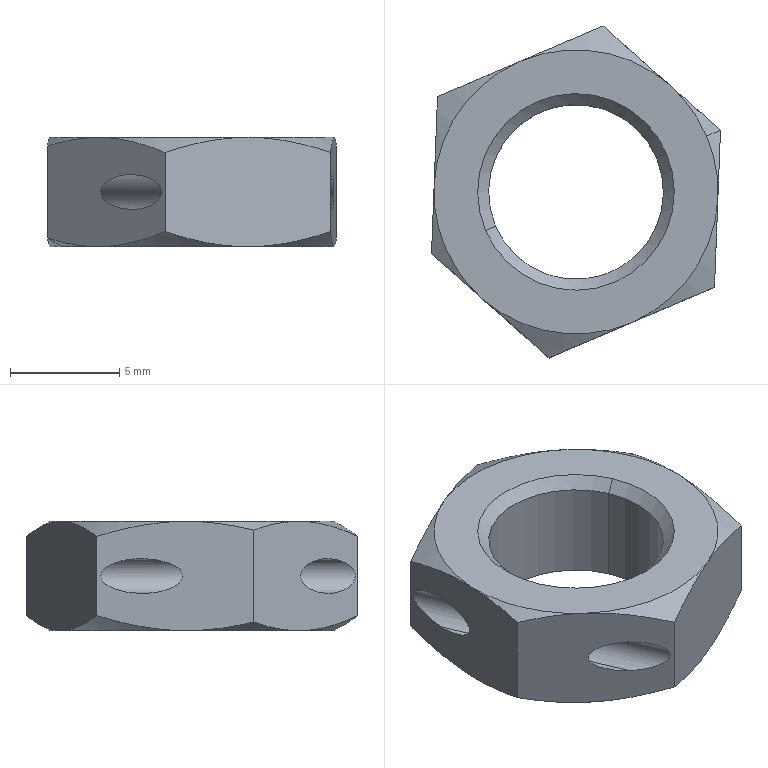Part | SolidWorks | features BaseBody 1 | 1 solid | 30 faces | box 13.225 x 15.189 x 5 mm | volume 437.577 mm3 | cone 16 | plane 8 | cylinder 6 | commonest cylinder face diameters 1.6 x4 8 x2
STEP:
#1=CARTESIAN_POINT('',(8.515,30.449,-145.05));
#2=VERTEX_POINT('',#1);
#3=CARTESIAN_POINT('',(6.902,32.713,-145.05));
#4=VERTEX_POINT('',#3);
#5=CARTESIAN_POINT('',(2.537,27.896,-145.05));
#6=DIRECTION('',(0.,0.,1.));
#7=DIRECTION('',(-0.9196,-0.3927,0.));
#8=AXIS2_PLACEMENT_3D('',#5,#6,#7);
#9=CIRCLE('',#8,6.5);
#10=EDGE_CURVE('',#2,#4,#9,.T.);
#11=ORIENTED_EDGE('',*,*,#10,.F.);
#12=CARTESIAN_POINT('',(9.149,30.72,-145.448));
#13=VERTEX_POINT('',#12);
#14=CARTESIAN_POINT('',(8.515,30.449,-145.05));
#15=DIRECTION('',(0.7964,0.3401,-0.5));
#16=VECTOR('',#15,1000.);
#17=LINE('',#14,#16);
#18=EDGE_CURVE('',#2,#13,#17,.T.);
#19=ORIENTED_EDGE('',*,*,#18,.T.);
#20=CARTESIAN_POINT('',(9.149,30.72,-145.448));
#21=CARTESIAN_POINT('',(8.411,31.375,-145.205));
#22=CARTESIAN_POINT('',(7.664,32.038,-145.056));
#23=CARTESIAN_POINT('',(6.902,32.713,-145.05));
#24=B_SPLINE_CURVE_WITH_KNOTS('',3,(#20,#21,#22,#23),.UNSPECIFIED.,.F.,.F.,(4,4),(0.,0.00303),.UNSPECIFIED.);
#25=EDGE_CURVE('',#13,#4,#24,.T.);
#26=ORIENTED_EDGE('',*,*,#25,.T.);
#27=EDGE_LOOP('',(#11,#19,#26));
#28=FACE_OUTER_BOUND('',#27,.T.);
#29=CARTESIAN_POINT('',(2.537,27.896,-145.05));
#30=DIRECTION('',(0.,0.,-1.));
#31=DIRECTION('',(0.9196,0.3927,0.));
#32=AXIS2_PLACEMENT_3D('',#29,#30,#31);
#33=CONICAL_SURFACE('',#32,6.5,1.047);
#34=ADVANCED_FACE('',(#28),#33,.T.);
#35=CARTESIAN_POINT('',(-3.958,28.144,-150.05));
#36=VERTEX_POINT('',#35);
#37=CARTESIAN_POINT('',(-3.441,25.343,-150.05));
#38=VERTEX_POINT('',#37);
#39=CARTESIAN_POINT('',(2.537,27.896,-150.05));
#40=DIRECTION('',(0.,0.,1.));
#41=DIRECTION('',(-0.9196,-0.3927,0.));
#42=AXIS2_PLACEMENT_3D('',#39,#40,#41);
#43=CIRCLE('',#42,6.5);
#44=EDGE_CURVE('',#36,#38,#43,.T.);
#45=ORIENTED_EDGE('',*,*,#44,.T.);
#46=CARTESIAN_POINT('',(-4.075,25.072,-149.652));
#47=VERTEX_POINT('',#46);
#48=CARTESIAN_POINT('',(-3.441,25.343,-150.05));
#49=DIRECTION('',(-0.7964,-0.3401,0.5));
#50=VECTOR('',#49,1000.);
#51=LINE('',#48,#50);
#52=EDGE_CURVE('',#38,#47,#51,.T.);
#53=ORIENTED_EDGE('',*,*,#52,.T.);
#54=CARTESIAN_POINT('',(-4.075,25.072,-149.652));
#55=CARTESIAN_POINT('',(-4.037,26.081,-149.901));
#56=CARTESIAN_POINT('',(-3.998,27.103,-150.05));
#57=CARTESIAN_POINT('',(-3.958,28.144,-150.05));
#58=B_SPLINE_CURVE_WITH_KNOTS('',3,(#54,#55,#56,#57),.UNSPECIFIED.,.F.,.F.,(4,4),(0.,0.003099),.UNSPECIFIED.);
#59=EDGE_CURVE('',#47,#36,#58,.T.);
#60=ORIENTED_EDGE('',*,*,#59,.T.);
#61=EDGE_LOOP('',(#45,#53,#60));
#62=FACE_OUTER_BOUND('',#61,.T.);
#63=CARTESIAN_POINT('',(2.537,27.896,-150.05));
#64=DIRECTION('',(0.,0.,1.));
#65=DIRECTION('',(-0.9196,-0.3927,0.));
#66=AXIS2_PLACEMENT_3D('',#63,#64,#65);
#67=CONICAL_SURFACE('',#66,6.5,1.047);
#68=ADVANCED_FACE('',(#62),#67,.T.);
#69=CARTESIAN_POINT('',(6.216,29.467,-150.05));
#70=VERTEX_POINT('',#69);
#71=CARTESIAN_POINT('',(-1.141,26.325,-150.05));
#72=VERTEX_POINT('',#71);
#73=CARTESIAN_POINT('',(2.537,27.896,-150.05));
#74=DIRECTION('',(0.,0.,-1.));
#75=DIRECTION('',(-0.9196,-0.3927,0.));
#76=AXIS2_PLACEMENT_3D('',#73,#74,#75);
#77=CIRCLE('',#76,4.);
#78=EDGE_CURVE('',#70,#72,#77,.T.);
#79=ORIENTED_EDGE('',*,*,#78,.T.);
#80=CARTESIAN_POINT('',(-1.141,26.325,-145.55));
#81=VERTEX_POINT('',#80);
#82=CARTESIAN_POINT('',(-1.141,26.325,-155.05));
#83=DIRECTION('',(0.,0.,1.));
#84=VECTOR('',#83,1000.);
#85=LINE('',#82,#84);
#86=EDGE_CURVE('',#72,#81,#85,.T.);
#87=ORIENTED_EDGE('',*,*,#86,.T.);
#88=CARTESIAN_POINT('',(6.216,29.467,-145.55));
#89=VERTEX_POINT('',#88);
#90=CARTESIAN_POINT('',(2.537,27.896,-145.55));
#91=DIRECTION('',(0.,0.,1.));
#92=DIRECTION('',(-0.9196,-0.3927,0.));
#93=AXIS2_PLACEMENT_3D('',#90,#91,#92);
#94=CIRCLE('',#93,4.);
#95=EDGE_CURVE('',#81,#89,#94,.T.);
#96=ORIENTED_EDGE('',*,*,#95,.T.);
#97=CARTESIAN_POINT('',(6.216,29.467,-155.05));
#98=DIRECTION('',(0.,0.,1.));
#99=VECTOR('',#98,1000.);
#100=LINE('',#97,#99);
#101=EDGE_CURVE('',#70,#89,#100,.T.);
#102=ORIENTED_EDGE('',*,*,#101,.F.);
#103=EDGE_LOOP('',(#79,#87,#96,#102));
#104=FACE_OUTER_BOUND('',#103,.T.);
#105=CARTESIAN_POINT('',(2.537,27.896,-155.05));
#106=DIRECTION('',(0.,0.,1.));
#107=DIRECTION('',(0.9196,0.3927,0.));
#108=AXIS2_PLACEMENT_3D('',#105,#106,#107);
#109=CYLINDRICAL_SURFACE('',#108,4.);
#110=ADVANCED_FACE('',(#104),#109,.F.);
#111=ORIENTED_EDGE('',*,*,#95,.F.);
#112=CARTESIAN_POINT('',(-1.601,26.129,-145.05));
#113=VERTEX_POINT('',#112);
#114=CARTESIAN_POINT('',(-1.141,26.325,-145.55));
#115=DIRECTION('',(-0.6503,-0.2777,0.7071));
#116=VECTOR('',#115,1000.);
#117=LINE('',#114,#116);
#118=EDGE_CURVE('',#81,#113,#117,.T.);
#119=ORIENTED_EDGE('',*,*,#118,.T.);
#120=CARTESIAN_POINT('',(6.676,29.664,-145.05));
#121=VERTEX_POINT('',#120);
#122=CARTESIAN_POINT('',(2.537,27.896,-145.05));
#123=DIRECTION('',(0.,0.,-1.));
#124=DIRECTION('',(-0.9196,-0.3927,0.));
#125=AXIS2_PLACEMENT_3D('',#122,#123,#124);
#126=CIRCLE('',#125,4.5);
#127=EDGE_CURVE('',#121,#113,#126,.T.);
#128=ORIENTED_EDGE('',*,*,#127,.F.);
#129=CARTESIAN_POINT('',(6.216,29.467,-145.55));
#130=DIRECTION('',(0.6503,0.2777,0.7071));
#131=VECTOR('',#130,1000.);
#132=LINE('',#129,#131);
#133=EDGE_CURVE('',#89,#121,#132,.T.);
#134=ORIENTED_EDGE('',*,*,#133,.F.);
#135=EDGE_LOOP('',(#111,#119,#128,#134));
#136=FACE_OUTER_BOUND('',#135,.T.);
#137=CARTESIAN_POINT('',(2.537,27.896,-145.55));
#138=DIRECTION('',(0.,0.,1.));
#139=DIRECTION('',(0.9196,0.3927,0.));
#140=AXIS2_PLACEMENT_3D('',#137,#138,#139);
#141=CONICAL_SURFACE('',#140,4.,0.7854);
#142=ADVANCED_FACE('',(#136),#141,.F.);
#143=CARTESIAN_POINT('',(8.954,25.601,-148.35));
#144=VERTEX_POINT('',#143);
#145=CARTESIAN_POINT('',(8.954,25.601,-146.75));
#146=VERTEX_POINT('',#145);
#147=CARTESIAN_POINT('',(8.954,25.601,-148.35));
#148=CARTESIAN_POINT('',(8.812,21.86,-148.35));
#149=CARTESIAN_POINT('',(8.812,21.86,-146.75));
#150=CARTESIAN_POINT('',(8.954,25.601,-146.75));
#151=(BOUNDED_CURVE()B_SPLINE_CURVE(3,(#147,#148,#149,#150),.UNSPECIFIED.,.F.,.F.)B_SPLINE_CURVE_WITH_KNOTS((4,4),(1.571,4.712),.UNSPECIFIED.)CURVE()GEOMETRIC_REPRESENTATION_ITEM()RATIONAL_B_SPLINE_CURVE((1.,0.3333,0.3333,1.))REPRESENTATION_ITEM(''));
#152=EDGE_CURVE('',#144,#146,#151,.T.);
#153=ORIENTED_EDGE('',*,*,#152,.F.);
#154=CARTESIAN_POINT('',(5.316,34.119,-148.35));
#155=VERTEX_POINT('',#154);
#156=CARTESIAN_POINT('',(9.688,23.882,-148.35));
#157=DIRECTION('',(-0.3927,0.9196,0.));
#158=VECTOR('',#157,1000.);
#159=LINE('',#156,#158);
#160=EDGE_CURVE('',#144,#155,#159,.T.);
#161=ORIENTED_EDGE('',*,*,#160,.T.);
#162=CARTESIAN_POINT('',(5.316,34.119,-146.75));
#163=VERTEX_POINT('',#162);
#164=CARTESIAN_POINT('',(5.316,34.119,-146.75));
#165=CARTESIAN_POINT('',(2.516,36.603,-146.75));
#166=CARTESIAN_POINT('',(2.516,36.603,-148.35));
#167=CARTESIAN_POINT('',(5.316,34.119,-148.35));
#168=(BOUNDED_CURVE()B_SPLINE_CURVE(3,(#164,#165,#166,#167),.UNSPECIFIED.,.F.,.F.)B_SPLINE_CURVE_WITH_KNOTS((4,4),(4.712,7.854),.UNSPECIFIED.)CURVE()GEOMETRIC_REPRESENTATION_ITEM()RATIONAL_B_SPLINE_CURVE((1.,0.3333,0.3333,1.))REPRESENTATION_ITEM(''));
#169=EDGE_CURVE('',#163,#155,#168,.T.);
#170=ORIENTED_EDGE('',*,*,#169,.F.);
#171=CARTESIAN_POINT('',(9.688,23.882,-146.75));
#172=DIRECTION('',(-0.3927,0.9196,0.));
#173=VECTOR('',#172,1000.);
#174=LINE('',#171,#173);
#175=EDGE_CURVE('',#146,#163,#174,.T.);
#176=ORIENTED_EDGE('',*,*,#175,.F.);
#177=EDGE_LOOP('',(#153,#161,#170,#176));
#178=FACE_OUTER_BOUND('',#177,.T.);
#179=CARTESIAN_POINT('',(9.688,23.882,-147.55));
#180=DIRECTION('',(-0.3927,0.9196,0.));
#181=DIRECTION('',(0.,0.,1.));
#182=AXIS2_PLACEMENT_3D('',#179,#180,#181);
#183=CYLINDRICAL_SURFACE('',#182,0.8);
#184=ADVANCED_FACE('',(#178),#183,.F.);
#185=CARTESIAN_POINT('',(-0.2421,21.673,-148.35));
#186=VERTEX_POINT('',#185);
#187=CARTESIAN_POINT('',(-0.2421,21.673,-146.75));
#188=VERTEX_POINT('',#187);
#189=CARTESIAN_POINT('',(-0.2421,21.673,-148.35));
#190=CARTESIAN_POINT('',(-3.042,24.157,-148.35));
#191=CARTESIAN_POINT('',(-3.042,24.157,-146.75));
#192=CARTESIAN_POINT('',(-0.2421,21.673,-146.75));
#193=(BOUNDED_CURVE()B_SPLINE_CURVE(3,(#189,#190,#191,#192),.UNSPECIFIED.,.F.,.F.)B_SPLINE_CURVE_WITH_KNOTS((4,4),(4.712,7.854),.UNSPECIFIED.)CURVE()GEOMETRIC_REPRESENTATION_ITEM()RATIONAL_B_SPLINE_CURVE((1.,0.3333,0.3333,1.))REPRESENTATION_ITEM(''));
#194=EDGE_CURVE('',#186,#188,#193,.T.);
#195=ORIENTED_EDGE('',*,*,#194,.F.);
#196=CARTESIAN_POINT('',(-3.88,30.192,-148.35));
#197=VERTEX_POINT('',#196);
#198=CARTESIAN_POINT('',(0.4917,19.955,-148.35));
#199=DIRECTION('',(-0.3927,0.9196,0.));
#200=VECTOR('',#199,1000.);
#201=LINE('',#198,#200);
#202=EDGE_CURVE('',#186,#197,#201,.T.);
#203=ORIENTED_EDGE('',*,*,#202,.T.);
#204=CARTESIAN_POINT('',(-3.88,30.192,-146.75));
#205=VERTEX_POINT('',#204);
#206=CARTESIAN_POINT('',(-3.88,30.192,-146.75));
#207=CARTESIAN_POINT('',(-4.023,26.452,-146.75));
#208=CARTESIAN_POINT('',(-4.023,26.452,-148.35));
#209=CARTESIAN_POINT('',(-3.88,30.192,-148.35));
#210=(BOUNDED_CURVE()B_SPLINE_CURVE(3,(#206,#207,#208,#209),.UNSPECIFIED.,.F.,.F.)B_SPLINE_CURVE_WITH_KNOTS((4,4),(1.571,4.712),.UNSPECIFIED.)CURVE()GEOMETRIC_REPRESENTATION_ITEM()RATIONAL_B_SPLINE_CURVE((1.,0.3333,0.3333,1.))REPRESENTATION_ITEM(''));
#211=EDGE_CURVE('',#205,#197,#210,.T.);
#212=ORIENTED_EDGE('',*,*,#211,.F.);
#213=CARTESIAN_POINT('',(0.4917,19.955,-146.75));
#214=DIRECTION('',(-0.3927,0.9196,0.));
#215=VECTOR('',#214,1000.);
#216=LINE('',#213,#215);
#217=EDGE_CURVE('',#188,#205,#216,.T.);
#218=ORIENTED_EDGE('',*,*,#217,.F.);
#219=EDGE_LOOP('',(#195,#203,#212,#218));
#220=FACE_OUTER_BOUND('',#219,.T.);
#221=CARTESIAN_POINT('',(0.4917,19.955,-147.55));
#222=DIRECTION('',(-0.3927,0.9196,0.));
#223=DIRECTION('',(0.,0.,1.));
#224=AXIS2_PLACEMENT_3D('',#221,#222,#223);
#225=CYLINDRICAL_SURFACE('',#224,0.8);
#226=ADVANCED_FACE('',(#220),#225,.F.);
#227=ORIENTED_EDGE('',*,*,#202,.F.);
#228=CARTESIAN_POINT('',(-0.2421,21.673,-146.75));
#229=CARTESIAN_POINT('',(2.558,19.19,-146.75));
#230=CARTESIAN_POINT('',(2.558,19.19,-148.35));
#231=CARTESIAN_POINT('',(-0.2421,21.673,-148.35));
#232=(BOUNDED_CURVE()B_SPLINE_CURVE(3,(#228,#229,#230,#231),.UNSPECIFIED.,.F.,.F.)B_SPLINE_CURVE_WITH_KNOTS((4,4),(1.571,4.712),.UNSPECIFIED.)CURVE()GEOMETRIC_REPRESENTATION_ITEM()RATIONAL_B_SPLINE_CURVE((1.,0.3333,0.3333,1.))REPRESENTATION_ITEM(''));
#233=EDGE_CURVE('',#188,#186,#232,.T.);
#234=ORIENTED_EDGE('',*,*,#233,.F.);
#235=ORIENTED_EDGE('',*,*,#217,.T.);
#236=CARTESIAN_POINT('',(-3.88,30.192,-148.35));
#237=CARTESIAN_POINT('',(-3.738,33.932,-148.35));
#238=CARTESIAN_POINT('',(-3.738,33.932,-146.75));
#239=CARTESIAN_POINT('',(-3.88,30.192,-146.75));
#240=(BOUNDED_CURVE()B_SPLINE_CURVE(3,(#236,#237,#238,#239),.UNSPECIFIED.,.F.,.F.)B_SPLINE_CURVE_WITH_KNOTS((4,4),(4.712,7.854),.UNSPECIFIED.)CURVE()GEOMETRIC_REPRESENTATION_ITEM()RATIONAL_B_SPLINE_CURVE((1.,0.3333,0.3333,1.))REPRESENTATION_ITEM(''));
#241=EDGE_CURVE('',#197,#205,#240,.T.);
#242=ORIENTED_EDGE('',*,*,#241,.F.);
#243=EDGE_LOOP('',(#227,#234,#235,#242));
#244=FACE_OUTER_BOUND('',#243,.T.);
#245=CARTESIAN_POINT('',(0.4917,19.955,-147.55));
#246=DIRECTION('',(-0.3927,0.9196,0.));
#247=DIRECTION('',(0.,0.,1.));
#248=AXIS2_PLACEMENT_3D('',#245,#246,#247);
#249=CYLINDRICAL_SURFACE('',#248,0.8);
#250=ADVANCED_FACE('',(#244),#249,.F.);
#251=ORIENTED_EDGE('',*,*,#160,.F.);
#252=CARTESIAN_POINT('',(8.954,25.601,-146.75));
#253=CARTESIAN_POINT('',(9.097,29.341,-146.75));
#254=CARTESIAN_POINT('',(9.097,29.341,-148.35));
#255=CARTESIAN_POINT('',(8.954,25.601,-148.35));
#256=(BOUNDED_CURVE()B_SPLINE_CURVE(3,(#252,#253,#254,#255),.UNSPECIFIED.,.F.,.F.)B_SPLINE_CURVE_WITH_KNOTS((4,4),(4.712,7.854),.UNSPECIFIED.)CURVE()GEOMETRIC_REPRESENTATION_ITEM()RATIONAL_B_SPLINE_CURVE((1.,0.3333,0.3333,1.))REPRESENTATION_ITEM(''));
#257=EDGE_CURVE('',#146,#144,#256,.T.);
#258=ORIENTED_EDGE('',*,*,#257,.F.);
#259=ORIENTED_EDGE('',*,*,#175,.T.);
#260=CARTESIAN_POINT('',(5.316,34.119,-148.35));
#261=CARTESIAN_POINT('',(8.117,31.636,-148.35));
#262=CARTESIAN_POINT('',(8.117,31.636,-146.75));
#263=CARTESIAN_POINT('',(5.316,34.119,-146.75));
#264=(BOUNDED_CURVE()B_SPLINE_CURVE(3,(#260,#261,#262,#263),.UNSPECIFIED.,.F.,.F.)B_SPLINE_CURVE_WITH_KNOTS((4,4),(1.571,4.712),.UNSPECIFIED.)CURVE()GEOMETRIC_REPRESENTATION_ITEM()RATIONAL_B_SPLINE_CURVE((1.,0.3333,0.3333,1.))REPRESENTATION_ITEM(''));
#265=EDGE_CURVE('',#155,#163,#264,.T.);
#266=ORIENTED_EDGE('',*,*,#265,.F.);
#267=EDGE_LOOP('',(#251,#258,#259,#266));
#268=FACE_OUTER_BOUND('',#267,.T.);
#269=CARTESIAN_POINT('',(9.688,23.882,-147.55));
#270=DIRECTION('',(-0.3927,0.9196,0.));
#271=DIRECTION('',(0.,0.,1.));
#272=AXIS2_PLACEMENT_3D('',#269,#270,#271);
#273=CYLINDRICAL_SURFACE('',#272,0.8);
#274=ADVANCED_FACE('',(#268),#273,.F.);
#275=ORIENTED_EDGE('',*,*,#118,.F.);
#276=CARTESIAN_POINT('',(2.537,27.896,-145.55));
#277=DIRECTION('',(0.,0.,1.));
#278=DIRECTION('',(-0.9196,-0.3927,0.));
#279=AXIS2_PLACEMENT_3D('',#276,#277,#278);
#280=CIRCLE('',#279,4.);
#281=EDGE_CURVE('',#89,#81,#280,.T.);
#282=ORIENTED_EDGE('',*,*,#281,.F.);
#283=ORIENTED_EDGE('',*,*,#133,.T.);
#284=CARTESIAN_POINT('',(2.537,27.896,-145.05));
#285=DIRECTION('',(0.,0.,-1.));
#286=DIRECTION('',(-0.9196,-0.3927,0.));
#287=AXIS2_PLACEMENT_3D('',#284,#285,#286);
#288=CIRCLE('',#287,4.5);
#289=EDGE_CURVE('',#113,#121,#288,.T.);
#290=ORIENTED_EDGE('',*,*,#289,.F.);
#291=EDGE_LOOP('',(#275,#282,#283,#290));
#292=FACE_OUTER_BOUND('',#291,.T.);
#293=CARTESIAN_POINT('',(2.537,27.896,-145.55));
#294=DIRECTION('',(0.,0.,1.));
#295=DIRECTION('',(0.9196,0.3927,0.));
#296=AXIS2_PLACEMENT_3D('',#293,#294,#295);
#297=CONICAL_SURFACE('',#296,4.,0.7854);
#298=ADVANCED_FACE('',(#292),#297,.F.);
#299=ORIENTED_EDGE('',*,*,#86,.F.);
#300=CARTESIAN_POINT('',(2.537,27.896,-150.05));
#301=DIRECTION('',(0.,0.,-1.));
#302=DIRECTION('',(-0.9196,-0.3927,0.));
#303=AXIS2_PLACEMENT_3D('',#300,#301,#302);
#304=CIRCLE('',#303,4.);
#305=EDGE_CURVE('',#72,#70,#304,.T.);
#306=ORIENTED_EDGE('',*,*,#305,.T.);
#307=ORIENTED_EDGE('',*,*,#101,.T.);
#308=ORIENTED_EDGE('',*,*,#281,.T.);
#309=EDGE_LOOP('',(#299,#306,#307,#308));
#310=FACE_OUTER_BOUND('',#309,.T.);
#311=CARTESIAN_POINT('',(2.537,27.896,-155.05));
#312=DIRECTION('',(0.,0.,1.));
#313=DIRECTION('',(0.9196,0.3927,0.));
#314=AXIS2_PLACEMENT_3D('',#311,#312,#313);
#315=CYLINDRICAL_SURFACE('',#314,4.);
#316=ADVANCED_FACE('',(#310),#315,.F.);
#317=CARTESIAN_POINT('',(-1.776,23.033,-150.05));
#318=VERTEX_POINT('',#317);
#319=CARTESIAN_POINT('',(5.09,21.919,-150.05));
#320=VERTEX_POINT('',#319);
#321=CARTESIAN_POINT('',(2.537,27.896,-150.05));
#322=DIRECTION('',(0.,0.,1.));
#323=DIRECTION('',(-0.9196,-0.3927,0.));
#324=AXIS2_PLACEMENT_3D('',#321,#322,#323);
#325=CIRCLE('',#324,6.5);
#326=EDGE_CURVE('',#318,#320,#325,.T.);
#327=ORIENTED_EDGE('',*,*,#326,.F.);
#328=CARTESIAN_POINT('',(2.537,27.896,-150.05));
#329=DIRECTION('',(0.,0.,1.));
#330=DIRECTION('',(-0.9196,-0.3927,0.));
#331=AXIS2_PLACEMENT_3D('',#328,#329,#330);
#332=CIRCLE('',#331,6.5);
#333=EDGE_CURVE('',#38,#318,#332,.T.);
#334=ORIENTED_EDGE('',*,*,#333,.F.);
#335=ORIENTED_EDGE('',*,*,#44,.F.);
#336=CARTESIAN_POINT('',(-0.01572,33.874,-150.05));
#337=VERTEX_POINT('',#336);
#338=CARTESIAN_POINT('',(2.537,27.896,-150.05));
#339=DIRECTION('',(0.,0.,-1.));
#340=DIRECTION('',(-0.9196,-0.3927,0.));
#341=AXIS2_PLACEMENT_3D('',#338,#339,#340);
#342=CIRCLE('',#341,6.5);
#343=EDGE_CURVE('',#36,#337,#342,.T.);
#344=ORIENTED_EDGE('',*,*,#343,.T.);
#345=CARTESIAN_POINT('',(6.85,32.759,-150.05));
#346=VERTEX_POINT('',#345);
#347=CARTESIAN_POINT('',(2.537,27.896,-150.05));
#348=DIRECTION('',(0.,0.,1.));
#349=DIRECTION('',(-0.9196,-0.3927,0.));
#350=AXIS2_PLACEMENT_3D('',#347,#348,#349);
#351=CIRCLE('',#350,6.5);
#352=EDGE_CURVE('',#346,#337,#351,.T.);
#353=ORIENTED_EDGE('',*,*,#352,.F.);
#354=CARTESIAN_POINT('',(9.032,27.649,-150.05));
#355=VERTEX_POINT('',#354);
#356=CARTESIAN_POINT('',(2.537,27.896,-150.05));
#357=DIRECTION('',(0.,0.,1.));
#358=DIRECTION('',(-0.9196,-0.3927,0.));
#359=AXIS2_PLACEMENT_3D('',#356,#357,#358);
#360=CIRCLE('',#359,6.5);
#361=EDGE_CURVE('',#355,#346,#360,.T.);
#362=ORIENTED_EDGE('',*,*,#361,.F.);
#363=CARTESIAN_POINT('',(2.537,27.896,-150.05));
#364=DIRECTION('',(0.,0.,1.));
#365=DIRECTION('',(-0.9196,-0.3927,0.));
#366=AXIS2_PLACEMENT_3D('',#363,#364,#365);
#367=CIRCLE('',#366,6.5);
#368=EDGE_CURVE('',#320,#355,#367,.T.);
#369=ORIENTED_EDGE('',*,*,#368,.F.);
#370=EDGE_LOOP('',(#327,#334,#335,#344,#353,#362,#369));
#371=FACE_OUTER_BOUND('',#370,.T.);
#372=ORIENTED_EDGE('',*,*,#78,.F.);
#373=ORIENTED_EDGE('',*,*,#305,.F.);
#374=EDGE_LOOP('',(#372,#373));
#375=FACE_BOUND('',#374,.T.);
#376=CARTESIAN_POINT('',(9.423,37.905,-150.05));
#377=DIRECTION('',(0.,0.,-1.));
#378=DIRECTION('',(0.,-1.,0.));
#379=AXIS2_PLACEMENT_3D('',#376,#377,#378);
#380=PLANE('',#379);
#381=ADVANCED_FACE('',(#371,#375),#380,.T.);
#382=CARTESIAN_POINT('',(1.304,20.302,-149.361));
#383=VERTEX_POINT('',#382);
#384=CARTESIAN_POINT('',(1.304,20.302,-149.361));
#385=CARTESIAN_POINT('',(0.8024,20.747,-149.568));
#386=CARTESIAN_POINT('',(0.2964,21.195,-149.741));
#387=CARTESIAN_POINT('',(-0.7287,22.105,-149.983));
#388=CARTESIAN_POINT('',(-1.248,22.565,-150.05));
#389=CARTESIAN_POINT('',(-1.776,23.033,-150.05));
#390=B_SPLINE_CURVE_WITH_KNOTS('',3,(#384,#385,#386,#387,#388,#389),.UNSPECIFIED.,.F.,.F.,(4,2,4),(0.,0.002087,0.004174),.UNSPECIFIED.);
#391=EDGE_CURVE('',#383,#318,#390,.T.);
#392=ORIENTED_EDGE('',*,*,#391,.T.);
#393=ORIENTED_EDGE('',*,*,#326,.T.);
#394=CARTESIAN_POINT('',(5.09,21.919,-150.05));
#395=CARTESIAN_POINT('',(4.441,21.641,-150.05));
#396=CARTESIAN_POINT('',(3.803,21.369,-149.983));
#397=CARTESIAN_POINT('',(2.543,20.831,-149.741));
#398=CARTESIAN_POINT('',(1.921,20.565,-149.568));
#399=CARTESIAN_POINT('',(1.304,20.302,-149.361));
#400=B_SPLINE_CURVE_WITH_KNOTS('',3,(#394,#395,#396,#397,#398,#399),.UNSPECIFIED.,.F.,.F.,(4,2,4),(0.,0.002087,0.004174),.UNSPECIFIED.);
#401=EDGE_CURVE('',#320,#383,#400,.T.);
#402=ORIENTED_EDGE('',*,*,#401,.T.);
#403=EDGE_LOOP('',(#392,#393,#402));
#404=FACE_OUTER_BOUND('',#403,.T.);
#405=CARTESIAN_POINT('',(2.537,27.896,-150.05));
#406=DIRECTION('',(0.,0.,1.));
#407=DIRECTION('',(-0.9196,-0.3927,0.));
#408=AXIS2_PLACEMENT_3D('',#405,#406,#407);
#409=CONICAL_SURFACE('',#408,6.5,1.047);
#410=ADVANCED_FACE('',(#404),#409,.T.);
#411=CARTESIAN_POINT('',(8.876,23.535,-149.361));
#412=VERTEX_POINT('',#411);
#413=CARTESIAN_POINT('',(9.032,27.649,-150.05));
#414=CARTESIAN_POINT('',(9.006,26.944,-150.05));
#415=CARTESIAN_POINT('',(8.979,26.25,-149.983));
#416=CARTESIAN_POINT('',(8.927,24.881,-149.741));
#417=CARTESIAN_POINT('',(8.901,24.205,-149.568));
#418=CARTESIAN_POINT('',(8.876,23.535,-149.361));
#419=B_SPLINE_CURVE_WITH_KNOTS('',3,(#413,#414,#415,#416,#417,#418),.UNSPECIFIED.,.F.,.F.,(4,2,4),(0.,0.002087,0.004174),.UNSPECIFIED.);
#420=EDGE_CURVE('',#355,#412,#419,.T.);
#421=ORIENTED_EDGE('',*,*,#420,.T.);
#422=CARTESIAN_POINT('',(8.876,23.535,-149.361));
#423=CARTESIAN_POINT('',(8.259,23.272,-149.568));
#424=CARTESIAN_POINT('',(7.637,23.006,-149.741));
#425=CARTESIAN_POINT('',(6.377,22.468,-149.983));
#426=CARTESIAN_POINT('',(5.739,22.196,-150.05));
#427=CARTESIAN_POINT('',(5.09,21.919,-150.05));
#428=B_SPLINE_CURVE_WITH_KNOTS('',3,(#422,#423,#424,#425,#426,#427),.UNSPECIFIED.,.F.,.F.,(4,2,4),(0.,0.002087,0.004174),.UNSPECIFIED.);
#429=EDGE_CURVE('',#412,#320,#428,.T.);
#430=ORIENTED_EDGE('',*,*,#429,.T.);
#431=ORIENTED_EDGE('',*,*,#368,.T.);
#432=EDGE_LOOP('',(#421,#430,#431));
#433=FACE_OUTER_BOUND('',#432,.T.);
#434=CARTESIAN_POINT('',(2.537,27.896,-150.05));
#435=DIRECTION('',(0.,0.,1.));
#436=DIRECTION('',(-0.9196,-0.3927,0.));
#437=AXIS2_PLACEMENT_3D('',#434,#435,#436);
#438=CONICAL_SURFACE('',#437,6.5,1.047);
#439=ADVANCED_FACE('',(#433),#438,.T.);
#440=CARTESIAN_POINT('',(9.149,30.72,-149.652));
#441=VERTEX_POINT('',#440);
#442=CARTESIAN_POINT('',(6.85,32.759,-150.05));
#443=CARTESIAN_POINT('',(7.629,32.068,-150.05));
#444=CARTESIAN_POINT('',(8.394,31.39,-149.901));
#445=CARTESIAN_POINT('',(9.149,30.72,-149.652));
#446=B_SPLINE_CURVE_WITH_KNOTS('',3,(#442,#443,#444,#445),.UNSPECIFIED.,.F.,.F.,(4,4),(0.,0.003099),.UNSPECIFIED.);
#447=EDGE_CURVE('',#346,#441,#446,.T.);
#448=ORIENTED_EDGE('',*,*,#447,.T.);
#449=CARTESIAN_POINT('',(9.149,30.72,-149.652));
#450=CARTESIAN_POINT('',(9.111,29.711,-149.901));
#451=CARTESIAN_POINT('',(9.072,28.69,-150.05));
#452=CARTESIAN_POINT('',(9.032,27.649,-150.05));
#453=B_SPLINE_CURVE_WITH_KNOTS('',3,(#449,#450,#451,#452),.UNSPECIFIED.,.F.,.F.,(4,4),(0.,0.003099),.UNSPECIFIED.);
#454=EDGE_CURVE('',#441,#355,#453,.T.);
#455=ORIENTED_EDGE('',*,*,#454,.T.);
#456=ORIENTED_EDGE('',*,*,#361,.T.);
#457=EDGE_LOOP('',(#448,#455,#456));
#458=FACE_OUTER_BOUND('',#457,.T.);
#459=CARTESIAN_POINT('',(2.537,27.896,-150.05));
#460=DIRECTION('',(0.,0.,1.));
#461=DIRECTION('',(-0.9196,-0.3927,0.));
#462=AXIS2_PLACEMENT_3D('',#459,#460,#461);
#463=CONICAL_SURFACE('',#462,6.5,1.047);
#464=ADVANCED_FACE('',(#458),#463,.T.);
#465=CARTESIAN_POINT('',(3.77,35.491,-149.361));
#466=VERTEX_POINT('',#465);
#467=CARTESIAN_POINT('',(-0.01572,33.874,-150.05));
#468=CARTESIAN_POINT('',(0.6329,34.151,-150.05));
#469=CARTESIAN_POINT('',(1.271,34.424,-149.983));
#470=CARTESIAN_POINT('',(2.531,34.962,-149.741));
#471=CARTESIAN_POINT('',(3.153,35.227,-149.568));
#472=CARTESIAN_POINT('',(3.77,35.491,-149.361));
#473=B_SPLINE_CURVE_WITH_KNOTS('',3,(#467,#468,#469,#470,#471,#472),.UNSPECIFIED.,.F.,.F.,(4,2,4),(0.,0.002087,0.004174),.UNSPECIFIED.);
#474=EDGE_CURVE('',#337,#466,#473,.T.);
#475=ORIENTED_EDGE('',*,*,#474,.T.);
#476=CARTESIAN_POINT('',(3.77,35.491,-149.361));
#477=CARTESIAN_POINT('',(4.272,35.046,-149.568));
#478=CARTESIAN_POINT('',(4.778,34.597,-149.741));
#479=CARTESIAN_POINT('',(5.803,33.688,-149.983));
#480=CARTESIAN_POINT('',(6.322,33.227,-150.05));
#481=CARTESIAN_POINT('',(6.85,32.759,-150.05));
#482=B_SPLINE_CURVE_WITH_KNOTS('',3,(#476,#477,#478,#479,#480,#481),.UNSPECIFIED.,.F.,.F.,(4,2,4),(0.,0.002087,0.004174),.UNSPECIFIED.);
#483=EDGE_CURVE('',#466,#346,#482,.T.);
#484=ORIENTED_EDGE('',*,*,#483,.T.);
#485=ORIENTED_EDGE('',*,*,#352,.T.);
#486=EDGE_LOOP('',(#475,#484,#485));
#487=FACE_OUTER_BOUND('',#486,.T.);
#488=CARTESIAN_POINT('',(2.537,27.896,-150.05));
#489=DIRECTION('',(0.,0.,1.));
#490=DIRECTION('',(-0.9196,-0.3927,0.));
#491=AXIS2_PLACEMENT_3D('',#488,#489,#490);
#492=CONICAL_SURFACE('',#491,6.5,1.047);
#493=ADVANCED_FACE('',(#487),#492,.T.);
#494=CARTESIAN_POINT('',(-3.801,32.257,-149.361));
#495=VERTEX_POINT('',#494);
#496=CARTESIAN_POINT('',(-3.801,32.257,-149.361));
#497=CARTESIAN_POINT('',(-3.185,32.521,-149.568));
#498=CARTESIAN_POINT('',(-2.563,32.786,-149.741));
#499=CARTESIAN_POINT('',(-1.303,33.324,-149.983));
#500=CARTESIAN_POINT('',(-0.6644,33.597,-150.05));
#501=CARTESIAN_POINT('',(-0.01572,33.874,-150.05));
#502=B_SPLINE_CURVE_WITH_KNOTS('',3,(#496,#497,#498,#499,#500,#501),.UNSPECIFIED.,.F.,.F.,(4,2,4),(0.,0.002087,0.004174),.UNSPECIFIED.);
#503=EDGE_CURVE('',#495,#337,#502,.T.);
#504=ORIENTED_EDGE('',*,*,#503,.T.);
#505=ORIENTED_EDGE('',*,*,#343,.F.);
#506=CARTESIAN_POINT('',(-3.958,28.144,-150.05));
#507=CARTESIAN_POINT('',(-3.931,28.848,-150.05));
#508=CARTESIAN_POINT('',(-3.905,29.542,-149.983));
#509=CARTESIAN_POINT('',(-3.853,30.911,-149.741));
#510=CARTESIAN_POINT('',(-3.827,31.587,-149.568));
#511=CARTESIAN_POINT('',(-3.801,32.257,-149.361));
#512=B_SPLINE_CURVE_WITH_KNOTS('',3,(#506,#507,#508,#509,#510,#511),.UNSPECIFIED.,.F.,.F.,(4,2,4),(0.,0.002087,0.004174),.UNSPECIFIED.);
#513=EDGE_CURVE('',#36,#495,#512,.T.);
#514=ORIENTED_EDGE('',*,*,#513,.T.);
#515=EDGE_LOOP('',(#504,#505,#514));
#516=FACE_OUTER_BOUND('',#515,.T.);
#517=CARTESIAN_POINT('',(2.537,27.896,-150.05));
#518=DIRECTION('',(0.,0.,1.));
#519=DIRECTION('',(-0.9196,-0.3927,0.));
#520=AXIS2_PLACEMENT_3D('',#517,#518,#519);
#521=CONICAL_SURFACE('',#520,6.5,1.047);
#522=ADVANCED_FACE('',(#516),#521,.T.);
#523=ORIENTED_EDGE('',*,*,#52,.F.);
#524=ORIENTED_EDGE('',*,*,#333,.T.);
#525=CARTESIAN_POINT('',(-1.776,23.033,-150.05));
#526=CARTESIAN_POINT('',(-2.555,23.724,-150.05));
#527=CARTESIAN_POINT('',(-3.32,24.403,-149.901));
#528=CARTESIAN_POINT('',(-4.075,25.072,-149.652));
#529=B_SPLINE_CURVE_WITH_KNOTS('',3,(#525,#526,#527,#528),.UNSPECIFIED.,.F.,.F.,(4,4),(0.,0.003099),.UNSPECIFIED.);
#530=EDGE_CURVE('',#318,#47,#529,.T.);
#531=ORIENTED_EDGE('',*,*,#530,.T.);
#532=EDGE_LOOP('',(#523,#524,#531));
#533=FACE_OUTER_BOUND('',#532,.T.);
#534=CARTESIAN_POINT('',(2.537,27.896,-150.05));
#535=DIRECTION('',(0.,0.,1.));
#536=DIRECTION('',(-0.9196,-0.3927,0.));
#537=AXIS2_PLACEMENT_3D('',#534,#535,#536);
#538=CONICAL_SURFACE('',#537,6.5,1.047);
#539=ADVANCED_FACE('',(#533),#538,.T.);
#540=CARTESIAN_POINT('',(-1.723,22.987,-145.05));
#541=VERTEX_POINT('',#540);
#542=CARTESIAN_POINT('',(1.304,20.302,-145.739));
#543=VERTEX_POINT('',#542);
#544=CARTESIAN_POINT('',(-1.723,22.987,-145.05));
#545=CARTESIAN_POINT('',(-0.686,22.067,-145.059));
#546=CARTESIAN_POINT('',(0.3177,21.177,-145.332));
#547=CARTESIAN_POINT('',(1.304,20.302,-145.739));
#548=B_SPLINE_CURVE_WITH_KNOTS('',3,(#544,#545,#546,#547),.UNSPECIFIED.,.F.,.F.,(4,4),(0.,0.004105),.UNSPECIFIED.);
#549=EDGE_CURVE('',#541,#543,#548,.T.);
#550=ORIENTED_EDGE('',*,*,#549,.T.);
#551=CARTESIAN_POINT('',(5.026,21.891,-145.05));
#552=VERTEX_POINT('',#551);
#553=CARTESIAN_POINT('',(1.304,20.302,-145.739));
#554=CARTESIAN_POINT('',(2.517,20.82,-145.332));
#555=CARTESIAN_POINT('',(3.751,21.346,-145.059));
#556=CARTESIAN_POINT('',(5.026,21.891,-145.05));
#557=B_SPLINE_CURVE_WITH_KNOTS('',3,(#553,#554,#555,#556),.UNSPECIFIED.,.F.,.F.,(4,4),(0.,0.004105),.UNSPECIFIED.);
#558=EDGE_CURVE('',#543,#552,#557,.T.);
#559=ORIENTED_EDGE('',*,*,#558,.T.);
#560=CARTESIAN_POINT('',(2.537,27.896,-145.05));
#561=DIRECTION('',(0.,0.,1.));
#562=DIRECTION('',(-0.9196,-0.3927,0.));
#563=AXIS2_PLACEMENT_3D('',#560,#561,#562);
#564=CIRCLE('',#563,6.5);
#565=EDGE_CURVE('',#541,#552,#564,.T.);
#566=ORIENTED_EDGE('',*,*,#565,.F.);
#567=EDGE_LOOP('',(#550,#559,#566));
#568=FACE_OUTER_BOUND('',#567,.T.);
#569=CARTESIAN_POINT('',(2.537,27.896,-145.05));
#570=DIRECTION('',(0.,0.,-1.));
#571=DIRECTION('',(0.9196,0.3927,0.));
#572=AXIS2_PLACEMENT_3D('',#569,#570,#571);
#573=CONICAL_SURFACE('',#572,6.5,1.047);
#574=ADVANCED_FACE('',(#568),#573,.T.);
#575=CARTESIAN_POINT('',(8.876,23.535,-145.739));
#576=VERTEX_POINT('',#575);
#577=CARTESIAN_POINT('',(9.03,27.579,-145.05));
#578=VERTEX_POINT('',#577);
#579=CARTESIAN_POINT('',(8.876,23.535,-145.739));
#580=CARTESIAN_POINT('',(8.926,24.853,-145.332));
#581=CARTESIAN_POINT('',(8.977,26.193,-145.059));
#582=CARTESIAN_POINT('',(9.03,27.579,-145.05));
#583=B_SPLINE_CURVE_WITH_KNOTS('',3,(#579,#580,#581,#582),.UNSPECIFIED.,.F.,.F.,(4,4),(0.,0.004105),.UNSPECIFIED.);
#584=EDGE_CURVE('',#576,#578,#583,.T.);
#585=ORIENTED_EDGE('',*,*,#584,.T.);
#586=CARTESIAN_POINT('',(5.154,21.946,-145.05));
#587=VERTEX_POINT('',#586);
#588=CARTESIAN_POINT('',(2.537,27.896,-145.05));
#589=DIRECTION('',(0.,0.,1.));
#590=DIRECTION('',(-0.9196,-0.3927,0.));
#591=AXIS2_PLACEMENT_3D('',#588,#589,#590);
#592=CIRCLE('',#591,6.5);
#593=EDGE_CURVE('',#587,#578,#592,.T.);
#594=ORIENTED_EDGE('',*,*,#593,.F.);
#595=CARTESIAN_POINT('',(5.154,21.946,-145.05));
#596=CARTESIAN_POINT('',(6.429,22.491,-145.059));
#597=CARTESIAN_POINT('',(7.663,23.017,-145.332));
#598=CARTESIAN_POINT('',(8.876,23.535,-145.739));
#599=B_SPLINE_CURVE_WITH_KNOTS('',3,(#595,#596,#597,#598),.UNSPECIFIED.,.F.,.F.,(4,4),(0.,0.004105),.UNSPECIFIED.);
#600=EDGE_CURVE('',#587,#576,#599,.T.);
#601=ORIENTED_EDGE('',*,*,#600,.T.);
#602=EDGE_LOOP('',(#585,#594,#601));
#603=FACE_OUTER_BOUND('',#602,.T.);
#604=CARTESIAN_POINT('',(2.537,27.896,-145.05));
#605=DIRECTION('',(0.,0.,-1.));
#606=DIRECTION('',(0.9196,0.3927,0.));
#607=AXIS2_PLACEMENT_3D('',#604,#605,#606);
#608=CONICAL_SURFACE('',#607,6.5,1.047);
#609=ADVANCED_FACE('',(#603),#608,.T.);
#610=ORIENTED_EDGE('',*,*,#18,.F.);
#611=CARTESIAN_POINT('',(9.035,27.719,-145.05));
#612=VERTEX_POINT('',#611);
#613=CARTESIAN_POINT('',(2.537,27.896,-145.05));
#614=DIRECTION('',(0.,0.,1.));
#615=DIRECTION('',(-0.9196,-0.3927,0.));
#616=AXIS2_PLACEMENT_3D('',#613,#614,#615);
#617=CIRCLE('',#616,6.5);
#618=EDGE_CURVE('',#612,#2,#617,.T.);
#619=ORIENTED_EDGE('',*,*,#618,.F.);
#620=CARTESIAN_POINT('',(9.035,27.719,-145.05));
#621=CARTESIAN_POINT('',(9.074,28.736,-145.056));
#622=CARTESIAN_POINT('',(9.112,29.734,-145.205));
#623=CARTESIAN_POINT('',(9.149,30.72,-145.448));
#624=B_SPLINE_CURVE_WITH_KNOTS('',3,(#620,#621,#622,#623),.UNSPECIFIED.,.F.,.F.,(4,4),(0.,0.00303),.UNSPECIFIED.);
#625=EDGE_CURVE('',#612,#13,#624,.T.);
#626=ORIENTED_EDGE('',*,*,#625,.T.);
#627=EDGE_LOOP('',(#610,#619,#626));
#628=FACE_OUTER_BOUND('',#627,.T.);
#629=CARTESIAN_POINT('',(2.537,27.896,-145.05));
#630=DIRECTION('',(0.,0.,-1.));
#631=DIRECTION('',(0.9196,0.3927,0.));
#632=AXIS2_PLACEMENT_3D('',#629,#630,#631);
#633=CONICAL_SURFACE('',#632,6.5,1.047);
#634=ADVANCED_FACE('',(#628),#633,.T.);
#635=CARTESIAN_POINT('',(6.798,32.806,-145.05));
#636=VERTEX_POINT('',#635);
#637=CARTESIAN_POINT('',(3.77,35.491,-145.739));
#638=VERTEX_POINT('',#637);
#639=CARTESIAN_POINT('',(6.798,32.806,-145.05));
#640=CARTESIAN_POINT('',(5.76,33.726,-145.059));
#641=CARTESIAN_POINT('',(4.757,34.616,-145.332));
#642=CARTESIAN_POINT('',(3.77,35.491,-145.739));
#643=B_SPLINE_CURVE_WITH_KNOTS('',3,(#639,#640,#641,#642),.UNSPECIFIED.,.F.,.F.,(4,4),(0.,0.004105),.UNSPECIFIED.);
#644=EDGE_CURVE('',#636,#638,#643,.T.);
#645=ORIENTED_EDGE('',*,*,#644,.T.);
#646=CARTESIAN_POINT('',(0.04861,33.901,-145.05));
#647=VERTEX_POINT('',#646);
#648=CARTESIAN_POINT('',(3.77,35.491,-145.739));
#649=CARTESIAN_POINT('',(2.557,34.973,-145.332));
#650=CARTESIAN_POINT('',(1.324,34.446,-145.059));
#651=CARTESIAN_POINT('',(0.04861,33.901,-145.05));
#652=B_SPLINE_CURVE_WITH_KNOTS('',3,(#648,#649,#650,#651),.UNSPECIFIED.,.F.,.F.,(4,4),(0.,0.004105),.UNSPECIFIED.);
#653=EDGE_CURVE('',#638,#647,#652,.T.);
#654=ORIENTED_EDGE('',*,*,#653,.T.);
#655=CARTESIAN_POINT('',(2.537,27.896,-145.05));
#656=DIRECTION('',(0.,0.,1.));
#657=DIRECTION('',(-0.9196,-0.3927,0.));
#658=AXIS2_PLACEMENT_3D('',#655,#656,#657);
#659=CIRCLE('',#658,6.5);
#660=EDGE_CURVE('',#636,#647,#659,.T.);
#661=ORIENTED_EDGE('',*,*,#660,.F.);
#662=EDGE_LOOP('',(#645,#654,#661));
#663=FACE_OUTER_BOUND('',#662,.T.);
#664=CARTESIAN_POINT('',(2.537,27.896,-145.05));
#665=DIRECTION('',(0.,0.,-1.));
#666=DIRECTION('',(0.9196,0.3927,0.));
#667=AXIS2_PLACEMENT_3D('',#664,#665,#666);
#668=CONICAL_SURFACE('',#667,6.5,1.047);
#669=ADVANCED_FACE('',(#663),#668,.T.);
#670=CARTESIAN_POINT('',(-0.08005,33.846,-145.05));
#671=VERTEX_POINT('',#670);
#672=CARTESIAN_POINT('',(-3.801,32.257,-145.739));
#673=VERTEX_POINT('',#672);
#674=CARTESIAN_POINT('',(-0.08005,33.846,-145.05));
#675=CARTESIAN_POINT('',(-1.355,33.302,-145.059));
#676=CARTESIAN_POINT('',(-2.589,32.775,-145.332));
#677=CARTESIAN_POINT('',(-3.801,32.257,-145.739));
#678=B_SPLINE_CURVE_WITH_KNOTS('',3,(#674,#675,#676,#677),.UNSPECIFIED.,.F.,.F.,(4,4),(0.,0.004105),.UNSPECIFIED.);
#679=EDGE_CURVE('',#671,#673,#678,.T.);
#680=ORIENTED_EDGE('',*,*,#679,.T.);
#681=CARTESIAN_POINT('',(-3.956,28.214,-145.05));
#682=VERTEX_POINT('',#681);
#683=CARTESIAN_POINT('',(-3.801,32.257,-145.739));
#684=CARTESIAN_POINT('',(-3.852,30.94,-145.332));
#685=CARTESIAN_POINT('',(-3.903,29.599,-145.059));
#686=CARTESIAN_POINT('',(-3.956,28.214,-145.05));
#687=B_SPLINE_CURVE_WITH_KNOTS('',3,(#683,#684,#685,#686),.UNSPECIFIED.,.F.,.F.,(4,4),(0.,0.004105),.UNSPECIFIED.);
#688=EDGE_CURVE('',#673,#682,#687,.T.);
#689=ORIENTED_EDGE('',*,*,#688,.T.);
#690=CARTESIAN_POINT('',(2.537,27.896,-145.05));
#691=DIRECTION('',(0.,0.,1.));
#692=DIRECTION('',(-0.9196,-0.3927,0.));
#693=AXIS2_PLACEMENT_3D('',#690,#691,#692);
#694=CIRCLE('',#693,6.5);
#695=EDGE_CURVE('',#671,#682,#694,.T.);
#696=ORIENTED_EDGE('',*,*,#695,.F.);
#697=EDGE_LOOP('',(#680,#689,#696));
#698=FACE_OUTER_BOUND('',#697,.T.);
#699=CARTESIAN_POINT('',(2.537,27.896,-145.05));
#700=DIRECTION('',(0.,0.,-1.));
#701=DIRECTION('',(0.9196,0.3927,0.));
#702=AXIS2_PLACEMENT_3D('',#699,#700,#701);
#703=CONICAL_SURFACE('',#702,6.5,1.047);
#704=ADVANCED_FACE('',(#698),#703,.T.);
#705=CARTESIAN_POINT('',(-3.961,28.074,-145.05));
#706=VERTEX_POINT('',#705);
#707=CARTESIAN_POINT('',(-4.075,25.072,-145.448));
#708=VERTEX_POINT('',#707);
#709=CARTESIAN_POINT('',(-3.961,28.074,-145.05));
#710=CARTESIAN_POINT('',(-4.,27.057,-145.056));
#711=CARTESIAN_POINT('',(-4.038,26.058,-145.205));
#712=CARTESIAN_POINT('',(-4.075,25.072,-145.448));
#713=B_SPLINE_CURVE_WITH_KNOTS('',3,(#709,#710,#711,#712),.UNSPECIFIED.,.F.,.F.,(4,4),(0.,0.00303),.UNSPECIFIED.);
#714=EDGE_CURVE('',#706,#708,#713,.T.);
#715=ORIENTED_EDGE('',*,*,#714,.T.);
#716=CARTESIAN_POINT('',(-1.828,23.08,-145.05));
#717=VERTEX_POINT('',#716);
#718=CARTESIAN_POINT('',(-4.075,25.072,-145.448));
#719=CARTESIAN_POINT('',(-3.337,24.418,-145.205));
#720=CARTESIAN_POINT('',(-2.59,23.755,-145.056));
#721=CARTESIAN_POINT('',(-1.828,23.08,-145.05));
#722=B_SPLINE_CURVE_WITH_KNOTS('',3,(#718,#719,#720,#721),.UNSPECIFIED.,.F.,.F.,(4,4),(0.,0.00303),.UNSPECIFIED.);
#723=EDGE_CURVE('',#708,#717,#722,.T.);
#724=ORIENTED_EDGE('',*,*,#723,.T.);
#725=CARTESIAN_POINT('',(2.537,27.896,-145.05));
#726=DIRECTION('',(0.,0.,1.));
#727=DIRECTION('',(-0.9196,-0.3927,0.));
#728=AXIS2_PLACEMENT_3D('',#725,#726,#727);
#729=CIRCLE('',#728,6.5);
#730=EDGE_CURVE('',#706,#717,#729,.T.);
#731=ORIENTED_EDGE('',*,*,#730,.F.);
#732=EDGE_LOOP('',(#715,#724,#731));
#733=FACE_OUTER_BOUND('',#732,.T.);
#734=CARTESIAN_POINT('',(2.537,27.896,-145.05));
#735=DIRECTION('',(0.,0.,-1.));
#736=DIRECTION('',(0.9196,0.3927,0.));
#737=AXIS2_PLACEMENT_3D('',#734,#735,#736);
#738=CONICAL_SURFACE('',#737,6.5,1.047);
#739=ADVANCED_FACE('',(#733),#738,.T.);
#740=CARTESIAN_POINT('',(1.304,20.302,-145.05));
#741=DIRECTION('',(0.7482,-0.6635,0.));
#742=VECTOR('',#741,1000.);
#743=LINE('',#740,#742);
#744=EDGE_CURVE('',#717,#541,#743,.T.);
#745=ORIENTED_EDGE('',*,*,#744,.T.);
#746=ORIENTED_EDGE('',*,*,#565,.T.);
#747=CARTESIAN_POINT('',(1.304,20.302,-145.05));
#748=DIRECTION('',(0.9196,0.3927,0.));
#749=VECTOR('',#748,1000.);
#750=LINE('',#747,#749);
#751=EDGE_CURVE('',#552,#587,#750,.T.);
#752=ORIENTED_EDGE('',*,*,#751,.T.);
#753=ORIENTED_EDGE('',*,*,#593,.T.);
#754=CARTESIAN_POINT('',(8.876,23.535,-145.05));
#755=DIRECTION('',(0.03806,0.9993,0.));
#756=VECTOR('',#755,1000.);
#757=LINE('',#754,#756);
#758=EDGE_CURVE('',#578,#612,#757,.T.);
#759=ORIENTED_EDGE('',*,*,#758,.T.);
#760=ORIENTED_EDGE('',*,*,#618,.T.);
#761=ORIENTED_EDGE('',*,*,#10,.T.);
#762=CARTESIAN_POINT('',(3.77,35.491,-145.05));
#763=DIRECTION('',(-0.7482,0.6635,0.));
#764=VECTOR('',#763,1000.);
#765=LINE('',#762,#764);
#766=EDGE_CURVE('',#4,#636,#765,.T.);
#767=ORIENTED_EDGE('',*,*,#766,.T.);
#768=ORIENTED_EDGE('',*,*,#660,.T.);
#769=CARTESIAN_POINT('',(-3.801,32.257,-145.05));
#770=DIRECTION('',(-0.9196,-0.3927,0.));
#771=VECTOR('',#770,1000.);
#772=LINE('',#769,#771);
#773=EDGE_CURVE('',#647,#671,#772,.T.);
#774=ORIENTED_EDGE('',*,*,#773,.T.);
#775=ORIENTED_EDGE('',*,*,#695,.T.);
#776=CARTESIAN_POINT('',(-3.801,32.257,-145.05));
#777=DIRECTION('',(-0.03806,-0.9993,0.));
#778=VECTOR('',#777,1000.);
#779=LINE('',#776,#778);
#780=EDGE_CURVE('',#682,#706,#779,.T.);
#781=ORIENTED_EDGE('',*,*,#780,.T.);
#782=ORIENTED_EDGE('',*,*,#730,.T.);
#783=EDGE_LOOP('',(#745,#746,#752,#753,#759,#760,#761,#767,#768,#774,#775,#781,#782));
#784=FACE_OUTER_BOUND('',#783,.T.);
#785=ORIENTED_EDGE('',*,*,#127,.T.);
#786=ORIENTED_EDGE('',*,*,#289,.T.);
#787=EDGE_LOOP('',(#785,#786));
#788=FACE_BOUND('',#787,.T.);
#789=CARTESIAN_POINT('',(9.423,37.905,-145.05));
#790=DIRECTION('',(0.,0.,-1.));
#791=DIRECTION('',(0.,-1.,0.));
#792=AXIS2_PLACEMENT_3D('',#789,#790,#791);
#793=PLANE('',#792);
#794=ADVANCED_FACE('',(#784,#788),#793,.F.);
#795=ORIENTED_EDGE('',*,*,#429,.F.);
#796=CARTESIAN_POINT('',(8.876,23.535,-145.05));
#797=DIRECTION('',(0.,0.,-1.));
#798=VECTOR('',#797,1000.);
#799=LINE('',#796,#798);
#800=EDGE_CURVE('',#576,#412,#799,.T.);
#801=ORIENTED_EDGE('',*,*,#800,.F.);
#802=ORIENTED_EDGE('',*,*,#600,.F.);
#803=ORIENTED_EDGE('',*,*,#751,.F.);
#804=ORIENTED_EDGE('',*,*,#558,.F.);
#805=CARTESIAN_POINT('',(1.304,20.302,-145.05));
#806=DIRECTION('',(0.,0.,-1.));
#807=VECTOR('',#806,1000.);
#808=LINE('',#805,#807);
#809=EDGE_CURVE('',#543,#383,#808,.T.);
#810=ORIENTED_EDGE('',*,*,#809,.T.);
#811=ORIENTED_EDGE('',*,*,#401,.F.);
#812=EDGE_LOOP('',(#795,#801,#802,#803,#804,#810,#811));
#813=FACE_OUTER_BOUND('',#812,.T.);
#814=CARTESIAN_POINT('',(1.304,20.302,-145.05));
#815=DIRECTION('',(-0.3927,0.9196,0.));
#816=DIRECTION('',(0.,0.,1.));
#817=AXIS2_PLACEMENT_3D('',#814,#815,#816);
#818=PLANE('',#817);
#819=ADVANCED_FACE('',(#813),#818,.F.);
#820=ORIENTED_EDGE('',*,*,#391,.F.);
#821=ORIENTED_EDGE('',*,*,#809,.F.);
#822=ORIENTED_EDGE('',*,*,#549,.F.);
#823=ORIENTED_EDGE('',*,*,#744,.F.);
#824=ORIENTED_EDGE('',*,*,#723,.F.);
#825=CARTESIAN_POINT('',(-4.075,25.072,-145.05));
#826=DIRECTION('',(0.,0.,-1.));
#827=VECTOR('',#826,1000.);
#828=LINE('',#825,#827);
#829=EDGE_CURVE('',#708,#47,#828,.T.);
#830=ORIENTED_EDGE('',*,*,#829,.T.);
#831=ORIENTED_EDGE('',*,*,#530,.F.);
#832=EDGE_LOOP('',(#820,#821,#822,#823,#824,#830,#831));
#833=FACE_OUTER_BOUND('',#832,.T.);
#834=ORIENTED_EDGE('',*,*,#233,.T.);
#835=ORIENTED_EDGE('',*,*,#194,.T.);
#836=EDGE_LOOP('',(#834,#835));
#837=FACE_BOUND('',#836,.T.);
#838=CARTESIAN_POINT('',(1.304,20.302,-145.05));
#839=DIRECTION('',(0.6635,0.7482,0.));
#840=DIRECTION('',(0.,0.,-1.));
#841=AXIS2_PLACEMENT_3D('',#838,#839,#840);
#842=PLANE('',#841);
#843=ADVANCED_FACE('',(#833,#837),#842,.F.);
#844=ORIENTED_EDGE('',*,*,#59,.F.);
#845=ORIENTED_EDGE('',*,*,#829,.F.);
#846=ORIENTED_EDGE('',*,*,#714,.F.);
#847=ORIENTED_EDGE('',*,*,#780,.F.);
#848=ORIENTED_EDGE('',*,*,#688,.F.);
#849=CARTESIAN_POINT('',(-3.801,32.257,-145.05));
#850=DIRECTION('',(0.,0.,-1.));
#851=VECTOR('',#850,1000.);
#852=LINE('',#849,#851);
#853=EDGE_CURVE('',#673,#495,#852,.T.);
#854=ORIENTED_EDGE('',*,*,#853,.T.);
#855=ORIENTED_EDGE('',*,*,#513,.F.);
#856=EDGE_LOOP('',(#844,#845,#846,#847,#848,#854,#855));
#857=FACE_OUTER_BOUND('',#856,.T.);
#858=ORIENTED_EDGE('',*,*,#211,.T.);
#859=ORIENTED_EDGE('',*,*,#241,.T.);
#860=EDGE_LOOP('',(#858,#859));
#861=FACE_BOUND('',#860,.T.);
#862=CARTESIAN_POINT('',(-3.801,32.257,-145.05));
#863=DIRECTION('',(0.9993,-0.03806,0.));
#864=DIRECTION('',(0.,0.,-1.));
#865=AXIS2_PLACEMENT_3D('',#862,#863,#864);
#866=PLANE('',#865);
#867=ADVANCED_FACE('',(#857,#861),#866,.F.);
#868=ORIENTED_EDGE('',*,*,#503,.F.);
#869=ORIENTED_EDGE('',*,*,#853,.F.);
#870=ORIENTED_EDGE('',*,*,#679,.F.);
#871=ORIENTED_EDGE('',*,*,#773,.F.);
#872=ORIENTED_EDGE('',*,*,#653,.F.);
#873=CARTESIAN_POINT('',(3.77,35.491,-145.05));
#874=DIRECTION('',(0.,0.,-1.));
#875=VECTOR('',#874,1000.);
#876=LINE('',#873,#875);
#877=EDGE_CURVE('',#638,#466,#876,.T.);
#878=ORIENTED_EDGE('',*,*,#877,.T.);
#879=ORIENTED_EDGE('',*,*,#474,.F.);
#880=EDGE_LOOP('',(#868,#869,#870,#871,#872,#878,#879));
#881=FACE_OUTER_BOUND('',#880,.T.);
#882=CARTESIAN_POINT('',(-3.801,32.257,-145.05));
#883=DIRECTION('',(0.3927,-0.9196,0.));
#884=DIRECTION('',(0.,0.,-1.));
#885=AXIS2_PLACEMENT_3D('',#882,#883,#884);
#886=PLANE('',#885);
#887=ADVANCED_FACE('',(#881),#886,.F.);
#888=ORIENTED_EDGE('',*,*,#483,.F.);
#889=ORIENTED_EDGE('',*,*,#877,.F.);
#890=ORIENTED_EDGE('',*,*,#644,.F.);
#891=ORIENTED_EDGE('',*,*,#766,.F.);
#892=ORIENTED_EDGE('',*,*,#25,.F.);
#893=CARTESIAN_POINT('',(9.149,30.72,-145.05));
#894=DIRECTION('',(0.,0.,-1.));
#895=VECTOR('',#894,1000.);
#896=LINE('',#893,#895);
#897=EDGE_CURVE('',#13,#441,#896,.T.);
#898=ORIENTED_EDGE('',*,*,#897,.T.);
#899=ORIENTED_EDGE('',*,*,#447,.F.);
#900=EDGE_LOOP('',(#888,#889,#890,#891,#892,#898,#899));
#901=FACE_OUTER_BOUND('',#900,.T.);
#902=ORIENTED_EDGE('',*,*,#169,.T.);
#903=ORIENTED_EDGE('',*,*,#265,.T.);
#904=EDGE_LOOP('',(#902,#903));
#905=FACE_BOUND('',#904,.T.);
#906=CARTESIAN_POINT('',(3.77,35.491,-145.05));
#907=DIRECTION('',(-0.6635,-0.7482,0.));
#908=DIRECTION('',(-0.7482,0.6635,0.));
#909=AXIS2_PLACEMENT_3D('',#906,#907,#908);
#910=PLANE('',#909);
#911=ADVANCED_FACE('',(#901,#905),#910,.F.);
#912=ORIENTED_EDGE('',*,*,#454,.F.);
#913=ORIENTED_EDGE('',*,*,#897,.F.);
#914=ORIENTED_EDGE('',*,*,#625,.F.);
#915=ORIENTED_EDGE('',*,*,#758,.F.);
#916=ORIENTED_EDGE('',*,*,#584,.F.);
#917=ORIENTED_EDGE('',*,*,#800,.T.);
#918=ORIENTED_EDGE('',*,*,#420,.F.);
#919=EDGE_LOOP('',(#912,#913,#914,#915,#916,#917,#918));
#920=FACE_OUTER_BOUND('',#919,.T.);
#921=ORIENTED_EDGE('',*,*,#257,.T.);
#922=ORIENTED_EDGE('',*,*,#152,.T.);
#923=EDGE_LOOP('',(#921,#922));
#924=FACE_BOUND('',#923,.T.);
#925=CARTESIAN_POINT('',(8.876,23.535,-145.05));
#926=DIRECTION('',(-0.9993,0.03806,0.));
#927=DIRECTION('',(0.,0.,1.));
#928=AXIS2_PLACEMENT_3D('',#925,#926,#927);
#929=PLANE('',#928);
#930=ADVANCED_FACE('',(#920,#924),#929,.F.);
#931=CLOSED_SHELL('',(#34,#68,#110,#142,#184,#226,#250,#274,#298,#316,#381,#410,#439,#464,#493,#522,#539,#574,#609,#634,#669,#704,#739,#794,#819,#843,#867,#887,#911,#930));
#932=MANIFOLD_SOLID_BREP('',#931);
#933=CARTESIAN_POINT('',(0.,0.,0.));
#934=DIRECTION('',(0.,0.,1.));
#935=DIRECTION('',(1.,0.,0.));
#936=AXIS2_PLACEMENT_3D('',#933,#934,#935);
#937=(LENGTH_UNIT()NAMED_UNIT(*)SI_UNIT(.MILLI.,.METRE.));
#938=UNCERTAINTY_MEASURE_WITH_UNIT(LENGTH_MEASURE(0.00001),#937,'','');
#939=(NAMED_UNIT(*)PLANE_ANGLE_UNIT()SI_UNIT($,.RADIAN.));
#940=(NAMED_UNIT(*)SI_UNIT($,.STERADIAN.)SOLID_ANGLE_UNIT());
#941=(GEOMETRIC_REPRESENTATION_CONTEXT(3)GLOBAL_UNCERTAINTY_ASSIGNED_CONTEXT((#938))GLOBAL_UNIT_ASSIGNED_CONTEXT((#937,#939,#940))REPRESENTATION_CONTEXT('',''));
#942=ADVANCED_BREP_SHAPE_REPRESENTATION('',(#932,#936),#941);